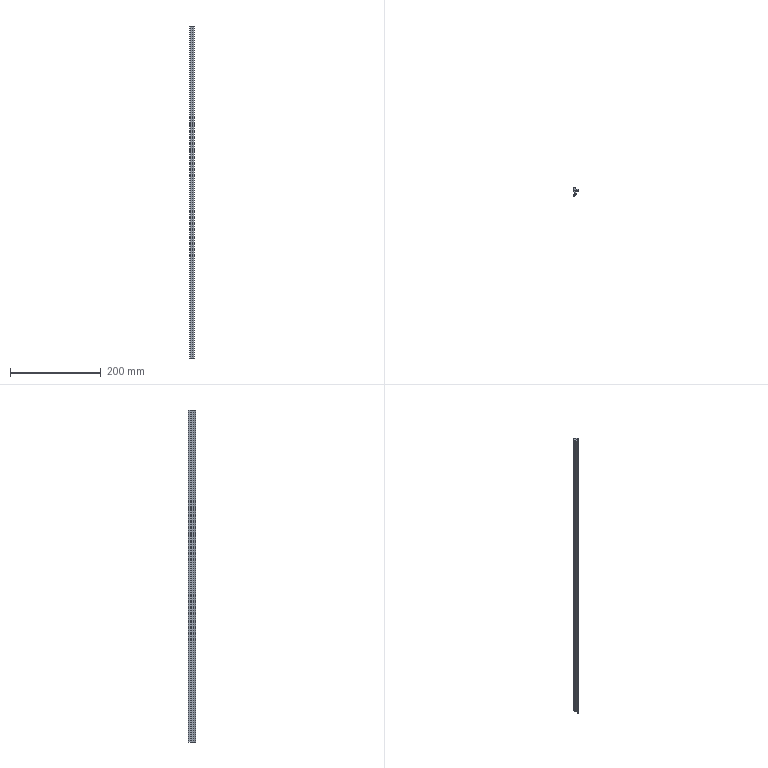Part | SolidWorks | features BaseBody 1, MoveFace 1 | 1 solid | 20 faces | box 10.8 x 17.5 x 730 mm | volume 57524 mm3 | cylinder 11 | plane 9 | commonest cylinder face diameters 1.6 x2 14 x2 0.4 x1 0.6 x1 0.8 x1 2.6 x1
STEP:
#1=CARTESIAN_POINT('',(-3.236,-11.055,630.));
#2=VERTEX_POINT('',#1);
#3=CARTESIAN_POINT('',(-4.3,-10.3,630.));
#4=VERTEX_POINT('',#3);
#5=CARTESIAN_POINT('',(-3.5,-10.3,630.));
#6=DIRECTION('',(0.,0.,-1.));
#7=DIRECTION('',(1.,0.,0.));
#8=AXIS2_PLACEMENT_3D('',#5,#6,#7);
#9=CIRCLE('',#8,0.8);
#10=EDGE_CURVE('',#2,#4,#9,.T.);
#11=ORIENTED_EDGE('',*,*,#10,.T.);
#12=CARTESIAN_POINT('',(-4.3,-10.3,-100.));
#13=VERTEX_POINT('',#12);
#14=CARTESIAN_POINT('',(-4.3,-10.3,-100.));
#15=DIRECTION('',(0.,0.,-1.));
#16=VECTOR('',#15,1000.);
#17=LINE('',#14,#16);
#18=EDGE_CURVE('',#4,#13,#17,.T.);
#19=ORIENTED_EDGE('',*,*,#18,.T.);
#20=CARTESIAN_POINT('',(-3.236,-11.055,-100.));
#21=VERTEX_POINT('',#20);
#22=CARTESIAN_POINT('',(-3.5,-10.3,-100.));
#23=DIRECTION('',(0.,0.,1.));
#24=DIRECTION('',(-1.,0.,0.));
#25=AXIS2_PLACEMENT_3D('',#22,#23,#24);
#26=CIRCLE('',#25,0.8);
#27=EDGE_CURVE('',#13,#21,#26,.T.);
#28=ORIENTED_EDGE('',*,*,#27,.T.);
#29=CARTESIAN_POINT('',(-3.236,-11.055,-100.));
#30=DIRECTION('',(0.,0.,-1.));
#31=VECTOR('',#30,1000.);
#32=LINE('',#29,#31);
#33=EDGE_CURVE('',#2,#21,#32,.T.);
#34=ORIENTED_EDGE('',*,*,#33,.F.);
#35=EDGE_LOOP('',(#11,#19,#28,#34));
#36=FACE_OUTER_BOUND('',#35,.T.);
#37=CARTESIAN_POINT('',(-3.5,-10.3,-100.));
#38=DIRECTION('',(0.,0.,-1.));
#39=DIRECTION('',(-1.,0.,0.));
#40=AXIS2_PLACEMENT_3D('',#37,#38,#39);
#41=CYLINDRICAL_SURFACE('',#40,0.8);
#42=ADVANCED_FACE('',(#36),#41,.T.);
#43=CARTESIAN_POINT('',(1.184,-6.397,-100.));
#44=VERTEX_POINT('',#43);
#45=CARTESIAN_POINT('',(-5.702,-4.29,-100.));
#46=DIRECTION('',(0.,0.,1.));
#47=DIRECTION('',(-1.,0.,0.));
#48=AXIS2_PLACEMENT_3D('',#45,#46,#47);
#49=CIRCLE('',#48,7.201);
#50=EDGE_CURVE('',#21,#44,#49,.T.);
#51=ORIENTED_EDGE('',*,*,#50,.T.);
#52=CARTESIAN_POINT('',(1.184,-6.397,630.));
#53=VERTEX_POINT('',#52);
#54=CARTESIAN_POINT('',(1.184,-6.397,-100.));
#55=DIRECTION('',(0.,0.,1.));
#56=VECTOR('',#55,1000.);
#57=LINE('',#54,#56);
#58=EDGE_CURVE('',#44,#53,#57,.T.);
#59=ORIENTED_EDGE('',*,*,#58,.T.);
#60=CARTESIAN_POINT('',(-5.702,-4.29,630.));
#61=DIRECTION('',(0.,0.,-1.));
#62=DIRECTION('',(1.,0.,0.));
#63=AXIS2_PLACEMENT_3D('',#60,#61,#62);
#64=CIRCLE('',#63,7.201);
#65=EDGE_CURVE('',#53,#2,#64,.T.);
#66=ORIENTED_EDGE('',*,*,#65,.T.);
#67=ORIENTED_EDGE('',*,*,#33,.T.);
#68=EDGE_LOOP('',(#51,#59,#66,#67));
#69=FACE_OUTER_BOUND('',#68,.T.);
#70=CARTESIAN_POINT('',(-5.702,-4.29,-100.));
#71=DIRECTION('',(0.,0.,-1.));
#72=DIRECTION('',(-1.,0.,0.));
#73=AXIS2_PLACEMENT_3D('',#70,#71,#72);
#74=CYLINDRICAL_SURFACE('',#73,7.201);
#75=ADVANCED_FACE('',(#69),#74,.T.);
#76=CARTESIAN_POINT('',(0.9,-6.,-100.));
#77=VERTEX_POINT('',#76);
#78=CARTESIAN_POINT('',(0.9,-6.3,-100.));
#79=DIRECTION('',(0.,0.,1.));
#80=DIRECTION('',(-1.,0.,0.));
#81=AXIS2_PLACEMENT_3D('',#78,#79,#80);
#82=CIRCLE('',#81,0.3);
#83=EDGE_CURVE('',#44,#77,#82,.T.);
#84=ORIENTED_EDGE('',*,*,#83,.T.);
#85=CARTESIAN_POINT('',(0.9,-6.,630.));
#86=VERTEX_POINT('',#85);
#87=CARTESIAN_POINT('',(0.9,-6.,-100.));
#88=DIRECTION('',(0.,0.,1.));
#89=VECTOR('',#88,1000.);
#90=LINE('',#87,#89);
#91=EDGE_CURVE('',#77,#86,#90,.T.);
#92=ORIENTED_EDGE('',*,*,#91,.T.);
#93=CARTESIAN_POINT('',(0.9,-6.3,630.));
#94=DIRECTION('',(0.,0.,-1.));
#95=DIRECTION('',(1.,0.,0.));
#96=AXIS2_PLACEMENT_3D('',#93,#94,#95);
#97=CIRCLE('',#96,0.3);
#98=EDGE_CURVE('',#86,#53,#97,.T.);
#99=ORIENTED_EDGE('',*,*,#98,.T.);
#100=ORIENTED_EDGE('',*,*,#58,.F.);
#101=EDGE_LOOP('',(#84,#92,#99,#100));
#102=FACE_OUTER_BOUND('',#101,.T.);
#103=CARTESIAN_POINT('',(0.9,-6.3,-100.));
#104=DIRECTION('',(0.,0.,-1.));
#105=DIRECTION('',(-1.,0.,0.));
#106=AXIS2_PLACEMENT_3D('',#103,#104,#105);
#107=CYLINDRICAL_SURFACE('',#106,0.3);
#108=ADVANCED_FACE('',(#102),#107,.T.);
#109=CARTESIAN_POINT('',(-2.5,-0.5,-100.));
#110=VERTEX_POINT('',#109);
#111=CARTESIAN_POINT('',(-2.5,-6.153,-100.));
#112=VERTEX_POINT('',#111);
#113=CARTESIAN_POINT('',(-2.5,-6.397,-100.));
#114=DIRECTION('',(0.,-1.,0.));
#115=VECTOR('',#114,1000.);
#116=LINE('',#113,#115);
#117=EDGE_CURVE('',#110,#112,#116,.T.);
#118=ORIENTED_EDGE('',*,*,#117,.F.);
#119=CARTESIAN_POINT('',(-4.2,1.695,-100.));
#120=VERTEX_POINT('',#119);
#121=CARTESIAN_POINT('',(-1.701,1.875,-100.));
#122=DIRECTION('',(0.,0.,1.));
#123=DIRECTION('',(-1.,0.,0.));
#124=AXIS2_PLACEMENT_3D('',#121,#122,#123);
#125=CIRCLE('',#124,2.506);
#126=EDGE_CURVE('',#120,#110,#125,.T.);
#127=ORIENTED_EDGE('',*,*,#126,.F.);
#128=CARTESIAN_POINT('',(-4.2,5.1,-100.));
#129=VERTEX_POINT('',#128);
#130=CARTESIAN_POINT('',(-4.2,-6.397,-100.));
#131=DIRECTION('',(0.,-1.,0.));
#132=VECTOR('',#131,1000.);
#133=LINE('',#130,#132);
#134=EDGE_CURVE('',#129,#120,#133,.T.);
#135=ORIENTED_EDGE('',*,*,#134,.F.);
#136=CARTESIAN_POINT('',(-2.892,6.4,-100.));
#137=VERTEX_POINT('',#136);
#138=CARTESIAN_POINT('',(-2.9,5.1,-100.));
#139=DIRECTION('',(0.,0.,1.));
#140=DIRECTION('',(-1.,0.,0.));
#141=AXIS2_PLACEMENT_3D('',#138,#139,#140);
#142=CIRCLE('',#141,1.3);
#143=EDGE_CURVE('',#137,#129,#142,.T.);
#144=ORIENTED_EDGE('',*,*,#143,.F.);
#145=CARTESIAN_POINT('',(0.5,5.5,-100.));
#146=VERTEX_POINT('',#145);
#147=CARTESIAN_POINT('',(-2.934,-0.5999,-100.));
#148=DIRECTION('',(0.,0.,1.));
#149=DIRECTION('',(-1.,0.,0.));
#150=AXIS2_PLACEMENT_3D('',#147,#148,#149);
#151=CIRCLE('',#150,7.);
#152=EDGE_CURVE('',#146,#137,#151,.T.);
#153=ORIENTED_EDGE('',*,*,#152,.F.);
#154=CARTESIAN_POINT('',(5.5,1.7,-100.));
#155=VERTEX_POINT('',#154);
#156=CARTESIAN_POINT('',(5.5,1.7,-100.));
#157=DIRECTION('',(-0.7962,0.6051,0.));
#158=VECTOR('',#157,1000.);
#159=LINE('',#156,#158);
#160=EDGE_CURVE('',#155,#146,#159,.T.);
#161=ORIENTED_EDGE('',*,*,#160,.F.);
#162=CARTESIAN_POINT('',(6.458,-0.2215,-100.));
#163=VERTEX_POINT('',#162);
#164=CARTESIAN_POINT('',(6.458,-0.2215,-100.));
#165=DIRECTION('',(-0.4462,0.8949,0.));
#166=VECTOR('',#165,1000.);
#167=LINE('',#164,#166);
#168=EDGE_CURVE('',#163,#155,#167,.T.);
#169=ORIENTED_EDGE('',*,*,#168,.F.);
#170=CARTESIAN_POINT('',(5.895,-0.7433,-100.));
#171=VERTEX_POINT('',#170);
#172=CARTESIAN_POINT('',(6.1,-0.4,-100.));
#173=DIRECTION('',(0.,0.,1.));
#174=DIRECTION('',(-1.,0.,0.));
#175=AXIS2_PLACEMENT_3D('',#172,#173,#174);
#176=CIRCLE('',#175,0.4);
#177=EDGE_CURVE('',#171,#163,#176,.T.);
#178=ORIENTED_EDGE('',*,*,#177,.F.);
#179=CARTESIAN_POINT('',(3.,0.,-100.));
#180=VERTEX_POINT('',#179);
#181=CARTESIAN_POINT('',(2.746,-6.995,-100.));
#182=DIRECTION('',(0.,0.,-1.));
#183=DIRECTION('',(-1.,0.,0.));
#184=AXIS2_PLACEMENT_3D('',#181,#182,#183);
#185=CIRCLE('',#184,7.);
#186=EDGE_CURVE('',#180,#171,#185,.T.);
#187=ORIENTED_EDGE('',*,*,#186,.F.);
#188=CARTESIAN_POINT('',(0.,0.,-100.));
#189=VERTEX_POINT('',#188);
#190=CARTESIAN_POINT('',(-6.814,0.,-100.));
#191=DIRECTION('',(1.,0.,0.));
#192=VECTOR('',#191,1000.);
#193=LINE('',#190,#192);
#194=EDGE_CURVE('',#189,#180,#193,.T.);
#195=ORIENTED_EDGE('',*,*,#194,.F.);
#196=CARTESIAN_POINT('',(0.,-5.8,-100.));
#197=VERTEX_POINT('',#196);
#198=CARTESIAN_POINT('',(0.,-6.397,-100.));
#199=DIRECTION('',(0.,1.,0.));
#200=VECTOR('',#199,1000.);
#201=LINE('',#198,#200);
#202=EDGE_CURVE('',#197,#189,#201,.T.);
#203=ORIENTED_EDGE('',*,*,#202,.F.);
#204=CARTESIAN_POINT('',(0.2,-6.,-100.));
#205=VERTEX_POINT('',#204);
#206=CARTESIAN_POINT('',(0.2,-5.8,-100.));
#207=DIRECTION('',(0.,0.,1.));
#208=DIRECTION('',(-1.,0.,0.));
#209=AXIS2_PLACEMENT_3D('',#206,#207,#208);
#210=CIRCLE('',#209,0.2);
#211=EDGE_CURVE('',#197,#205,#210,.T.);
#212=ORIENTED_EDGE('',*,*,#211,.T.);
#213=CARTESIAN_POINT('',(-6.814,-6.,-100.));
#214=DIRECTION('',(-1.,0.,0.));
#215=VECTOR('',#214,1000.);
#216=LINE('',#213,#215);
#217=EDGE_CURVE('',#77,#205,#216,.T.);
#218=ORIENTED_EDGE('',*,*,#217,.F.);
#219=ORIENTED_EDGE('',*,*,#83,.F.);
#220=ORIENTED_EDGE('',*,*,#50,.F.);
#221=ORIENTED_EDGE('',*,*,#27,.F.);
#222=CARTESIAN_POINT('',(-3.998,-9.674,-100.));
#223=VERTEX_POINT('',#222);
#224=CARTESIAN_POINT('',(-3.5,-10.3,-100.));
#225=DIRECTION('',(0.,0.,1.));
#226=DIRECTION('',(-1.,0.,0.));
#227=AXIS2_PLACEMENT_3D('',#224,#225,#226);
#228=CIRCLE('',#227,0.8);
#229=EDGE_CURVE('',#223,#13,#228,.T.);
#230=ORIENTED_EDGE('',*,*,#229,.F.);
#231=CARTESIAN_POINT('',(-6.814,-6.397,-100.));
#232=DIRECTION('',(0.,0.,-1.));
#233=DIRECTION('',(-1.,0.,0.));
#234=AXIS2_PLACEMENT_3D('',#231,#232,#233);
#235=CIRCLE('',#234,4.321);
#236=EDGE_CURVE('',#112,#223,#235,.T.);
#237=ORIENTED_EDGE('',*,*,#236,.F.);
#238=EDGE_LOOP('',(#118,#127,#135,#144,#153,#161,#169,#178,#187,#195,#203,#212,#218,#219,#220,#221,#230,#237));
#239=FACE_OUTER_BOUND('',#238,.T.);
#240=CARTESIAN_POINT('',(-6.814,-6.397,-100.));
#241=DIRECTION('',(0.,0.,1.));
#242=DIRECTION('',(1.,0.,0.));
#243=AXIS2_PLACEMENT_3D('',#240,#241,#242);
#244=PLANE('',#243);
#245=ADVANCED_FACE('',(#239),#244,.F.);
#246=ORIENTED_EDGE('',*,*,#18,.F.);
#247=CARTESIAN_POINT('',(-3.998,-9.674,630.));
#248=VERTEX_POINT('',#247);
#249=CARTESIAN_POINT('',(-3.5,-10.3,630.));
#250=DIRECTION('',(0.,0.,-1.));
#251=DIRECTION('',(1.,0.,0.));
#252=AXIS2_PLACEMENT_3D('',#249,#250,#251);
#253=CIRCLE('',#252,0.8);
#254=EDGE_CURVE('',#4,#248,#253,.T.);
#255=ORIENTED_EDGE('',*,*,#254,.T.);
#256=CARTESIAN_POINT('',(-3.998,-9.674,-100.));
#257=DIRECTION('',(0.,0.,-1.));
#258=VECTOR('',#257,1000.);
#259=LINE('',#256,#258);
#260=EDGE_CURVE('',#248,#223,#259,.T.);
#261=ORIENTED_EDGE('',*,*,#260,.T.);
#262=ORIENTED_EDGE('',*,*,#229,.T.);
#263=EDGE_LOOP('',(#246,#255,#261,#262));
#264=FACE_OUTER_BOUND('',#263,.T.);
#265=CARTESIAN_POINT('',(-3.5,-10.3,-100.));
#266=DIRECTION('',(0.,0.,-1.));
#267=DIRECTION('',(-1.,0.,0.));
#268=AXIS2_PLACEMENT_3D('',#265,#266,#267);
#269=CYLINDRICAL_SURFACE('',#268,0.8);
#270=ADVANCED_FACE('',(#264),#269,.T.);
#271=CARTESIAN_POINT('',(-4.2,1.695,630.));
#272=VERTEX_POINT('',#271);
#273=CARTESIAN_POINT('',(-2.5,-0.5,630.));
#274=VERTEX_POINT('',#273);
#275=CARTESIAN_POINT('',(-1.701,1.875,630.));
#276=DIRECTION('',(0.,0.,1.));
#277=DIRECTION('',(1.,0.,0.));
#278=AXIS2_PLACEMENT_3D('',#275,#276,#277);
#279=CIRCLE('',#278,2.506);
#280=EDGE_CURVE('',#272,#274,#279,.T.);
#281=ORIENTED_EDGE('',*,*,#280,.T.);
#282=CARTESIAN_POINT('',(-2.5,-6.153,630.));
#283=VERTEX_POINT('',#282);
#284=CARTESIAN_POINT('',(-2.5,-6.397,630.));
#285=DIRECTION('',(0.,-1.,0.));
#286=VECTOR('',#285,1000.);
#287=LINE('',#284,#286);
#288=EDGE_CURVE('',#274,#283,#287,.T.);
#289=ORIENTED_EDGE('',*,*,#288,.T.);
#290=CARTESIAN_POINT('',(-6.814,-6.397,630.));
#291=DIRECTION('',(0.,0.,-1.));
#292=DIRECTION('',(1.,0.,0.));
#293=AXIS2_PLACEMENT_3D('',#290,#291,#292);
#294=CIRCLE('',#293,4.321);
#295=EDGE_CURVE('',#283,#248,#294,.T.);
#296=ORIENTED_EDGE('',*,*,#295,.T.);
#297=ORIENTED_EDGE('',*,*,#254,.F.);
#298=ORIENTED_EDGE('',*,*,#10,.F.);
#299=ORIENTED_EDGE('',*,*,#65,.F.);
#300=ORIENTED_EDGE('',*,*,#98,.F.);
#301=CARTESIAN_POINT('',(0.2,-6.,630.));
#302=VERTEX_POINT('',#301);
#303=CARTESIAN_POINT('',(-6.814,-6.,630.));
#304=DIRECTION('',(-1.,0.,0.));
#305=VECTOR('',#304,1000.);
#306=LINE('',#303,#305);
#307=EDGE_CURVE('',#86,#302,#306,.T.);
#308=ORIENTED_EDGE('',*,*,#307,.T.);
#309=CARTESIAN_POINT('',(0.,-5.8,630.));
#310=VERTEX_POINT('',#309);
#311=CARTESIAN_POINT('',(0.2,-5.8,630.));
#312=DIRECTION('',(0.,0.,-1.));
#313=DIRECTION('',(1.,0.,0.));
#314=AXIS2_PLACEMENT_3D('',#311,#312,#313);
#315=CIRCLE('',#314,0.2);
#316=EDGE_CURVE('',#302,#310,#315,.T.);
#317=ORIENTED_EDGE('',*,*,#316,.T.);
#318=CARTESIAN_POINT('',(0.,0.,630.));
#319=VERTEX_POINT('',#318);
#320=CARTESIAN_POINT('',(0.,-6.397,630.));
#321=DIRECTION('',(0.,1.,0.));
#322=VECTOR('',#321,1000.);
#323=LINE('',#320,#322);
#324=EDGE_CURVE('',#310,#319,#323,.T.);
#325=ORIENTED_EDGE('',*,*,#324,.T.);
#326=CARTESIAN_POINT('',(3.,0.,630.));
#327=VERTEX_POINT('',#326);
#328=CARTESIAN_POINT('',(-6.814,0.,630.));
#329=DIRECTION('',(1.,0.,0.));
#330=VECTOR('',#329,1000.);
#331=LINE('',#328,#330);
#332=EDGE_CURVE('',#319,#327,#331,.T.);
#333=ORIENTED_EDGE('',*,*,#332,.T.);
#334=CARTESIAN_POINT('',(5.895,-0.7433,630.));
#335=VERTEX_POINT('',#334);
#336=CARTESIAN_POINT('',(2.746,-6.995,630.));
#337=DIRECTION('',(0.,0.,-1.));
#338=DIRECTION('',(1.,0.,0.));
#339=AXIS2_PLACEMENT_3D('',#336,#337,#338);
#340=CIRCLE('',#339,7.);
#341=EDGE_CURVE('',#327,#335,#340,.T.);
#342=ORIENTED_EDGE('',*,*,#341,.T.);
#343=CARTESIAN_POINT('',(6.458,-0.2215,630.));
#344=VERTEX_POINT('',#343);
#345=CARTESIAN_POINT('',(6.1,-0.4,630.));
#346=DIRECTION('',(0.,0.,-1.));
#347=DIRECTION('',(1.,0.,0.));
#348=AXIS2_PLACEMENT_3D('',#345,#346,#347);
#349=CIRCLE('',#348,0.4);
#350=EDGE_CURVE('',#344,#335,#349,.T.);
#351=ORIENTED_EDGE('',*,*,#350,.F.);
#352=CARTESIAN_POINT('',(5.5,1.7,630.));
#353=VERTEX_POINT('',#352);
#354=CARTESIAN_POINT('',(6.282,0.1323,630.));
#355=DIRECTION('',(-0.4462,0.8949,0.));
#356=VECTOR('',#355,1000.);
#357=LINE('',#354,#356);
#358=EDGE_CURVE('',#344,#353,#357,.T.);
#359=ORIENTED_EDGE('',*,*,#358,.T.);
#360=CARTESIAN_POINT('',(0.5,5.5,630.));
#361=VERTEX_POINT('',#360);
#362=CARTESIAN_POINT('',(1.595,4.668,630.));
#363=DIRECTION('',(-0.7962,0.6051,0.));
#364=VECTOR('',#363,1000.);
#365=LINE('',#362,#364);
#366=EDGE_CURVE('',#353,#361,#365,.T.);
#367=ORIENTED_EDGE('',*,*,#366,.T.);
#368=CARTESIAN_POINT('',(-2.892,6.4,630.));
#369=VERTEX_POINT('',#368);
#370=CARTESIAN_POINT('',(-2.934,-0.5999,630.));
#371=DIRECTION('',(0.,0.,1.));
#372=DIRECTION('',(1.,0.,0.));
#373=AXIS2_PLACEMENT_3D('',#370,#371,#372);
#374=CIRCLE('',#373,7.);
#375=EDGE_CURVE('',#361,#369,#374,.T.);
#376=ORIENTED_EDGE('',*,*,#375,.T.);
#377=CARTESIAN_POINT('',(-4.2,5.1,630.));
#378=VERTEX_POINT('',#377);
#379=CARTESIAN_POINT('',(-2.9,5.1,630.));
#380=DIRECTION('',(0.,0.,1.));
#381=DIRECTION('',(1.,0.,0.));
#382=AXIS2_PLACEMENT_3D('',#379,#380,#381);
#383=CIRCLE('',#382,1.3);
#384=EDGE_CURVE('',#369,#378,#383,.T.);
#385=ORIENTED_EDGE('',*,*,#384,.T.);
#386=CARTESIAN_POINT('',(-4.2,-6.397,630.));
#387=DIRECTION('',(0.,-1.,0.));
#388=VECTOR('',#387,1000.);
#389=LINE('',#386,#388);
#390=EDGE_CURVE('',#378,#272,#389,.T.);
#391=ORIENTED_EDGE('',*,*,#390,.T.);
#392=EDGE_LOOP('',(#281,#289,#296,#297,#298,#299,#300,#308,#317,#325,#333,#342,#351,#359,#367,#376,#385,#391));
#393=FACE_OUTER_BOUND('',#392,.T.);
#394=CARTESIAN_POINT('',(-6.814,-6.397,630.));
#395=DIRECTION('',(0.,0.,1.));
#396=DIRECTION('',(1.,0.,0.));
#397=AXIS2_PLACEMENT_3D('',#394,#395,#396);
#398=PLANE('',#397);
#399=ADVANCED_FACE('',(#393),#398,.T.);
#400=ORIENTED_EDGE('',*,*,#217,.T.);
#401=CARTESIAN_POINT('',(0.2,-6.,-100.));
#402=DIRECTION('',(0.,0.,1.));
#403=VECTOR('',#402,1000.);
#404=LINE('',#401,#403);
#405=EDGE_CURVE('',#205,#302,#404,.T.);
#406=ORIENTED_EDGE('',*,*,#405,.T.);
#407=ORIENTED_EDGE('',*,*,#307,.F.);
#408=ORIENTED_EDGE('',*,*,#91,.F.);
#409=EDGE_LOOP('',(#400,#406,#407,#408));
#410=FACE_OUTER_BOUND('',#409,.T.);
#411=CARTESIAN_POINT('',(0.9,-6.,-100.));
#412=DIRECTION('',(0.,1.,0.));
#413=DIRECTION('',(0.,0.,1.));
#414=AXIS2_PLACEMENT_3D('',#411,#412,#413);
#415=PLANE('',#414);
#416=ADVANCED_FACE('',(#410),#415,.T.);
#417=CARTESIAN_POINT('',(-2.5,-6.153,-100.));
#418=DIRECTION('',(0.,0.,1.));
#419=VECTOR('',#418,1000.);
#420=LINE('',#417,#419);
#421=EDGE_CURVE('',#112,#283,#420,.T.);
#422=ORIENTED_EDGE('',*,*,#421,.F.);
#423=ORIENTED_EDGE('',*,*,#236,.T.);
#424=ORIENTED_EDGE('',*,*,#260,.F.);
#425=ORIENTED_EDGE('',*,*,#295,.F.);
#426=EDGE_LOOP('',(#422,#423,#424,#425));
#427=FACE_OUTER_BOUND('',#426,.T.);
#428=CARTESIAN_POINT('',(-6.814,-6.397,-100.));
#429=DIRECTION('',(0.,0.,-1.));
#430=DIRECTION('',(-1.,0.,0.));
#431=AXIS2_PLACEMENT_3D('',#428,#429,#430);
#432=CYLINDRICAL_SURFACE('',#431,4.321);
#433=ADVANCED_FACE('',(#427),#432,.F.);
#434=ORIENTED_EDGE('',*,*,#117,.T.);
#435=ORIENTED_EDGE('',*,*,#421,.T.);
#436=ORIENTED_EDGE('',*,*,#288,.F.);
#437=CARTESIAN_POINT('',(-2.5,-0.5,-100.));
#438=DIRECTION('',(0.,0.,-1.));
#439=VECTOR('',#438,1000.);
#440=LINE('',#437,#439);
#441=EDGE_CURVE('',#274,#110,#440,.T.);
#442=ORIENTED_EDGE('',*,*,#441,.T.);
#443=EDGE_LOOP('',(#434,#435,#436,#442));
#444=FACE_OUTER_BOUND('',#443,.T.);
#445=CARTESIAN_POINT('',(-2.5,-0.5,-100.));
#446=DIRECTION('',(-1.,0.,0.));
#447=DIRECTION('',(0.,0.,1.));
#448=AXIS2_PLACEMENT_3D('',#445,#446,#447);
#449=PLANE('',#448);
#450=ADVANCED_FACE('',(#444),#449,.T.);
#451=ORIENTED_EDGE('',*,*,#126,.T.);
#452=ORIENTED_EDGE('',*,*,#441,.F.);
#453=ORIENTED_EDGE('',*,*,#280,.F.);
#454=CARTESIAN_POINT('',(-4.2,1.695,-100.));
#455=DIRECTION('',(0.,0.,-1.));
#456=VECTOR('',#455,1000.);
#457=LINE('',#454,#456);
#458=EDGE_CURVE('',#272,#120,#457,.T.);
#459=ORIENTED_EDGE('',*,*,#458,.T.);
#460=EDGE_LOOP('',(#451,#452,#453,#459));
#461=FACE_OUTER_BOUND('',#460,.T.);
#462=CARTESIAN_POINT('',(-1.701,1.875,-100.));
#463=DIRECTION('',(0.,0.,-1.));
#464=DIRECTION('',(-1.,0.,0.));
#465=AXIS2_PLACEMENT_3D('',#462,#463,#464);
#466=CYLINDRICAL_SURFACE('',#465,2.506);
#467=ADVANCED_FACE('',(#461),#466,.T.);
#468=ORIENTED_EDGE('',*,*,#134,.T.);
#469=ORIENTED_EDGE('',*,*,#458,.F.);
#470=ORIENTED_EDGE('',*,*,#390,.F.);
#471=CARTESIAN_POINT('',(-4.2,5.1,-100.));
#472=DIRECTION('',(0.,0.,-1.));
#473=VECTOR('',#472,1000.);
#474=LINE('',#471,#473);
#475=EDGE_CURVE('',#378,#129,#474,.T.);
#476=ORIENTED_EDGE('',*,*,#475,.T.);
#477=EDGE_LOOP('',(#468,#469,#470,#476));
#478=FACE_OUTER_BOUND('',#477,.T.);
#479=CARTESIAN_POINT('',(-4.2,5.1,-100.));
#480=DIRECTION('',(-1.,0.,0.));
#481=DIRECTION('',(0.,0.,1.));
#482=AXIS2_PLACEMENT_3D('',#479,#480,#481);
#483=PLANE('',#482);
#484=ADVANCED_FACE('',(#478),#483,.T.);
#485=ORIENTED_EDGE('',*,*,#143,.T.);
#486=ORIENTED_EDGE('',*,*,#475,.F.);
#487=ORIENTED_EDGE('',*,*,#384,.F.);
#488=CARTESIAN_POINT('',(-2.892,6.4,-100.));
#489=DIRECTION('',(0.,0.,-1.));
#490=VECTOR('',#489,1000.);
#491=LINE('',#488,#490);
#492=EDGE_CURVE('',#369,#137,#491,.T.);
#493=ORIENTED_EDGE('',*,*,#492,.T.);
#494=EDGE_LOOP('',(#485,#486,#487,#493));
#495=FACE_OUTER_BOUND('',#494,.T.);
#496=CARTESIAN_POINT('',(-2.9,5.1,-100.));
#497=DIRECTION('',(0.,0.,-1.));
#498=DIRECTION('',(-1.,0.,0.));
#499=AXIS2_PLACEMENT_3D('',#496,#497,#498);
#500=CYLINDRICAL_SURFACE('',#499,1.3);
#501=ADVANCED_FACE('',(#495),#500,.T.);
#502=ORIENTED_EDGE('',*,*,#152,.T.);
#503=ORIENTED_EDGE('',*,*,#492,.F.);
#504=ORIENTED_EDGE('',*,*,#375,.F.);
#505=CARTESIAN_POINT('',(0.5,5.5,-100.));
#506=DIRECTION('',(0.,0.,-1.));
#507=VECTOR('',#506,1000.);
#508=LINE('',#505,#507);
#509=EDGE_CURVE('',#361,#146,#508,.T.);
#510=ORIENTED_EDGE('',*,*,#509,.T.);
#511=EDGE_LOOP('',(#502,#503,#504,#510));
#512=FACE_OUTER_BOUND('',#511,.T.);
#513=CARTESIAN_POINT('',(-2.934,-0.5999,-100.));
#514=DIRECTION('',(0.,0.,-1.));
#515=DIRECTION('',(-1.,0.,0.));
#516=AXIS2_PLACEMENT_3D('',#513,#514,#515);
#517=CYLINDRICAL_SURFACE('',#516,7.);
#518=ADVANCED_FACE('',(#512),#517,.T.);
#519=ORIENTED_EDGE('',*,*,#160,.T.);
#520=ORIENTED_EDGE('',*,*,#509,.F.);
#521=ORIENTED_EDGE('',*,*,#366,.F.);
#522=CARTESIAN_POINT('',(5.5,1.7,-100.));
#523=DIRECTION('',(0.,0.,-1.));
#524=VECTOR('',#523,1000.);
#525=LINE('',#522,#524);
#526=EDGE_CURVE('',#353,#155,#525,.T.);
#527=ORIENTED_EDGE('',*,*,#526,.T.);
#528=EDGE_LOOP('',(#519,#520,#521,#527));
#529=FACE_OUTER_BOUND('',#528,.T.);
#530=CARTESIAN_POINT('',(5.5,1.7,-100.));
#531=DIRECTION('',(0.6051,0.7962,0.));
#532=DIRECTION('',(-0.7962,0.6051,0.));
#533=AXIS2_PLACEMENT_3D('',#530,#531,#532);
#534=PLANE('',#533);
#535=ADVANCED_FACE('',(#529),#534,.T.);
#536=ORIENTED_EDGE('',*,*,#168,.T.);
#537=ORIENTED_EDGE('',*,*,#526,.F.);
#538=ORIENTED_EDGE('',*,*,#358,.F.);
#539=CARTESIAN_POINT('',(6.458,-0.2215,-100.));
#540=DIRECTION('',(0.,0.,-1.));
#541=VECTOR('',#540,1000.);
#542=LINE('',#539,#541);
#543=EDGE_CURVE('',#344,#163,#542,.T.);
#544=ORIENTED_EDGE('',*,*,#543,.T.);
#545=EDGE_LOOP('',(#536,#537,#538,#544));
#546=FACE_OUTER_BOUND('',#545,.T.);
#547=CARTESIAN_POINT('',(6.458,-0.2215,-100.));
#548=DIRECTION('',(0.8949,0.4462,0.));
#549=DIRECTION('',(-0.4462,0.8949,0.));
#550=AXIS2_PLACEMENT_3D('',#547,#548,#549);
#551=PLANE('',#550);
#552=ADVANCED_FACE('',(#546),#551,.T.);
#553=CARTESIAN_POINT('',(3.,0.,-100.));
#554=DIRECTION('',(0.,0.,1.));
#555=VECTOR('',#554,1000.);
#556=LINE('',#553,#555);
#557=EDGE_CURVE('',#180,#327,#556,.T.);
#558=ORIENTED_EDGE('',*,*,#557,.F.);
#559=ORIENTED_EDGE('',*,*,#186,.T.);
#560=CARTESIAN_POINT('',(5.895,-0.7433,-100.));
#561=DIRECTION('',(0.,0.,-1.));
#562=VECTOR('',#561,1000.);
#563=LINE('',#560,#562);
#564=EDGE_CURVE('',#335,#171,#563,.T.);
#565=ORIENTED_EDGE('',*,*,#564,.F.);
#566=ORIENTED_EDGE('',*,*,#341,.F.);
#567=EDGE_LOOP('',(#558,#559,#565,#566));
#568=FACE_OUTER_BOUND('',#567,.T.);
#569=CARTESIAN_POINT('',(2.746,-6.995,-100.));
#570=DIRECTION('',(0.,0.,-1.));
#571=DIRECTION('',(-1.,0.,0.));
#572=AXIS2_PLACEMENT_3D('',#569,#570,#571);
#573=CYLINDRICAL_SURFACE('',#572,7.);
#574=ADVANCED_FACE('',(#568),#573,.F.);
#575=ORIENTED_EDGE('',*,*,#194,.T.);
#576=ORIENTED_EDGE('',*,*,#557,.T.);
#577=ORIENTED_EDGE('',*,*,#332,.F.);
#578=CARTESIAN_POINT('',(0.,0.,-100.));
#579=DIRECTION('',(0.,0.,-1.));
#580=VECTOR('',#579,1000.);
#581=LINE('',#578,#580);
#582=EDGE_CURVE('',#319,#189,#581,.T.);
#583=ORIENTED_EDGE('',*,*,#582,.T.);
#584=EDGE_LOOP('',(#575,#576,#577,#583));
#585=FACE_OUTER_BOUND('',#584,.T.);
#586=CARTESIAN_POINT('',(0.,0.,-100.));
#587=DIRECTION('',(0.,-1.,0.));
#588=DIRECTION('',(0.,0.,-1.));
#589=AXIS2_PLACEMENT_3D('',#586,#587,#588);
#590=PLANE('',#589);
#591=ADVANCED_FACE('',(#585),#590,.T.);
#592=ORIENTED_EDGE('',*,*,#202,.T.);
#593=ORIENTED_EDGE('',*,*,#582,.F.);
#594=ORIENTED_EDGE('',*,*,#324,.F.);
#595=CARTESIAN_POINT('',(0.,-5.8,-100.));
#596=DIRECTION('',(0.,0.,-1.));
#597=VECTOR('',#596,1000.);
#598=LINE('',#595,#597);
#599=EDGE_CURVE('',#310,#197,#598,.T.);
#600=ORIENTED_EDGE('',*,*,#599,.T.);
#601=EDGE_LOOP('',(#592,#593,#594,#600));
#602=FACE_OUTER_BOUND('',#601,.T.);
#603=CARTESIAN_POINT('',(0.,-5.8,-100.));
#604=DIRECTION('',(1.,0.,0.));
#605=DIRECTION('',(0.,0.,-1.));
#606=AXIS2_PLACEMENT_3D('',#603,#604,#605);
#607=PLANE('',#606);
#608=ADVANCED_FACE('',(#602),#607,.T.);
#609=ORIENTED_EDGE('',*,*,#405,.F.);
#610=ORIENTED_EDGE('',*,*,#211,.F.);
#611=ORIENTED_EDGE('',*,*,#599,.F.);
#612=ORIENTED_EDGE('',*,*,#316,.F.);
#613=EDGE_LOOP('',(#609,#610,#611,#612));
#614=FACE_OUTER_BOUND('',#613,.T.);
#615=CARTESIAN_POINT('',(0.2,-5.8,-100.));
#616=DIRECTION('',(0.,0.,-1.));
#617=DIRECTION('',(-1.,0.,0.));
#618=AXIS2_PLACEMENT_3D('',#615,#616,#617);
#619=CYLINDRICAL_SURFACE('',#618,0.2);
#620=ADVANCED_FACE('',(#614),#619,.F.);
#621=ORIENTED_EDGE('',*,*,#177,.T.);
#622=ORIENTED_EDGE('',*,*,#543,.F.);
#623=ORIENTED_EDGE('',*,*,#350,.T.);
#624=ORIENTED_EDGE('',*,*,#564,.T.);
#625=EDGE_LOOP('',(#621,#622,#623,#624));
#626=FACE_OUTER_BOUND('',#625,.T.);
#627=CARTESIAN_POINT('',(6.1,-0.4,-100.));
#628=DIRECTION('',(0.,0.,-1.));
#629=DIRECTION('',(-1.,0.,0.));
#630=AXIS2_PLACEMENT_3D('',#627,#628,#629);
#631=CYLINDRICAL_SURFACE('',#630,0.4);
#632=ADVANCED_FACE('',(#626),#631,.T.);
#633=CLOSED_SHELL('',(#42,#75,#108,#245,#270,#399,#416,#433,#450,#467,#484,#501,#518,#535,#552,#574,#591,#608,#620,#632));
#634=MANIFOLD_SOLID_BREP('',#633);
#635=CARTESIAN_POINT('',(0.,0.,0.));
#636=DIRECTION('',(0.,0.,1.));
#637=DIRECTION('',(1.,0.,0.));
#638=AXIS2_PLACEMENT_3D('',#635,#636,#637);
#639=(LENGTH_UNIT()NAMED_UNIT(*)SI_UNIT(.MILLI.,.METRE.));
#640=UNCERTAINTY_MEASURE_WITH_UNIT(LENGTH_MEASURE(0.00001),#639,'','');
#641=(NAMED_UNIT(*)PLANE_ANGLE_UNIT()SI_UNIT($,.RADIAN.));
#642=(NAMED_UNIT(*)SI_UNIT($,.STERADIAN.)SOLID_ANGLE_UNIT());
#643=(GEOMETRIC_REPRESENTATION_CONTEXT(3)GLOBAL_UNCERTAINTY_ASSIGNED_CONTEXT((#640))GLOBAL_UNIT_ASSIGNED_CONTEXT((#639,#641,#642))REPRESENTATION_CONTEXT('',''));
#644=ADVANCED_BREP_SHAPE_REPRESENTATION('',(#634,#638),#643);